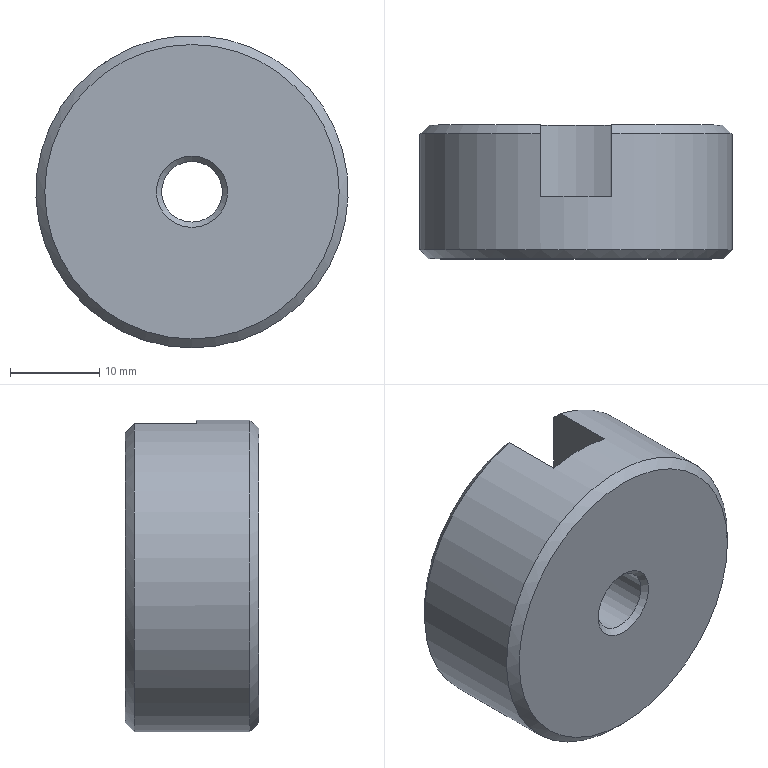Part | STEP file | 冲床-300配套压波_id598_x_t | 1 solid | 12 faces | box 35 x 15 x 35 mm | volume 11277 mm3 | plane 5 | cone 4 | cylinder 3 | commonest cylinder face diameters 6.8 x1 19 x1 35 x1
STEP:
#1=CARTESIAN_POINT('',(1396.,-127.,88.7));
#2=VERTEX_POINT('',#1);
#3=CARTESIAN_POINT('',(1388.,-127.,88.7));
#4=VERTEX_POINT('',#3);
#5=CARTESIAN_POINT('',(1392.,-127.,80.083));
#6=DIRECTION('',(0.,1.,0.));
#7=DIRECTION('',(0.,0.,-1.));
#8=AXIS2_PLACEMENT_3D('',#5,#6,#7);
#9=CIRCLE('',#8,9.5);
#10=EDGE_CURVE('',#2,#4,#9,.T.);
#11=ORIENTED_EDGE('',*,*,#10,.T.);
#12=CARTESIAN_POINT('',(1388.,-135.,88.7));
#13=VERTEX_POINT('',#12);
#14=CARTESIAN_POINT('',(1388.,-140.,88.7));
#15=DIRECTION('',(0.,-1.,0.));
#16=VECTOR('',#15,1.);
#17=LINE('',#14,#16);
#18=EDGE_CURVE('',#4,#13,#17,.T.);
#19=ORIENTED_EDGE('',*,*,#18,.T.);
#20=CARTESIAN_POINT('',(1396.,-135.,88.7));
#21=VERTEX_POINT('',#20);
#22=CARTESIAN_POINT('',(1392.,-135.,80.083));
#23=DIRECTION('',(0.,-1.,0.));
#24=DIRECTION('',(0.,0.,-1.));
#25=AXIS2_PLACEMENT_3D('',#22,#23,#24);
#26=CIRCLE('',#25,9.5);
#27=EDGE_CURVE('',#13,#21,#26,.T.);
#28=ORIENTED_EDGE('',*,*,#27,.T.);
#29=CARTESIAN_POINT('',(1396.,-140.,88.7));
#30=DIRECTION('',(0.,1.,0.));
#31=VECTOR('',#30,1.);
#32=LINE('',#29,#31);
#33=EDGE_CURVE('',#21,#2,#32,.T.);
#34=ORIENTED_EDGE('',*,*,#33,.T.);
#35=EDGE_LOOP('',(#11,#19,#28,#34));
#36=FACE_OUTER_BOUND('',#35,.T.);
#37=CARTESIAN_POINT('',(1392.,-140.,80.083));
#38=DIRECTION('',(0.,1.,0.));
#39=DIRECTION('',(-1.,0.,0.));
#40=AXIS2_PLACEMENT_3D('',#37,#38,#39);
#41=CYLINDRICAL_SURFACE('',#40,9.5);
#42=ADVANCED_FACE('',(#36),#41,.F.);
#43=CARTESIAN_POINT('',(1392.,-141.,62.583));
#44=VERTEX_POINT('',#43);
#45=CARTESIAN_POINT('',(1392.,-141.,80.083));
#46=DIRECTION('',(0.,1.,0.));
#47=DIRECTION('',(0.,0.,-1.));
#48=AXIS2_PLACEMENT_3D('',#45,#46,#47);
#49=CIRCLE('',#48,17.5);
#50=EDGE_CURVE('',#44,#44,#49,.T.);
#51=ORIENTED_EDGE('',*,*,#50,.T.);
#52=EDGE_LOOP('',(#51));
#53=FACE_BOUND('',#52,.T.);
#54=CARTESIAN_POINT('',(1388.,-128.,97.12));
#55=VERTEX_POINT('',#54);
#56=CARTESIAN_POINT('',(1388.,-135.,97.12));
#57=VERTEX_POINT('',#56);
#58=CARTESIAN_POINT('',(1388.,-142.,97.12));
#59=DIRECTION('',(0.,-1.,0.));
#60=VECTOR('',#59,1.);
#61=LINE('',#58,#60);
#62=EDGE_CURVE('',#55,#57,#61,.T.);
#63=ORIENTED_EDGE('',*,*,#62,.F.);
#64=CARTESIAN_POINT('',(1396.,-128.,97.12));
#65=VERTEX_POINT('',#64);
#66=CARTESIAN_POINT('',(1392.,-128.,80.083));
#67=DIRECTION('',(0.,-1.,0.));
#68=DIRECTION('',(0.,0.,-1.));
#69=AXIS2_PLACEMENT_3D('',#66,#67,#68);
#70=CIRCLE('',#69,17.5);
#71=EDGE_CURVE('',#55,#65,#70,.T.);
#72=ORIENTED_EDGE('',*,*,#71,.T.);
#73=CARTESIAN_POINT('',(1396.,-135.,97.12));
#74=VERTEX_POINT('',#73);
#75=CARTESIAN_POINT('',(1396.,-142.,97.12));
#76=DIRECTION('',(0.,1.,0.));
#77=VECTOR('',#76,1.);
#78=LINE('',#75,#77);
#79=EDGE_CURVE('',#74,#65,#78,.T.);
#80=ORIENTED_EDGE('',*,*,#79,.F.);
#81=CARTESIAN_POINT('',(1392.,-135.,80.083));
#82=DIRECTION('',(0.,-1.,0.));
#83=DIRECTION('',(0.,0.,1.));
#84=AXIS2_PLACEMENT_3D('',#81,#82,#83);
#85=CIRCLE('',#84,17.5);
#86=EDGE_CURVE('',#74,#57,#85,.T.);
#87=ORIENTED_EDGE('',*,*,#86,.T.);
#88=EDGE_LOOP('',(#63,#72,#80,#87));
#89=FACE_BOUND('',#88,.T.);
#90=CARTESIAN_POINT('',(1392.,-142.,80.083));
#91=DIRECTION('',(0.,1.,0.));
#92=DIRECTION('',(0.,0.,1.));
#93=AXIS2_PLACEMENT_3D('',#90,#91,#92);
#94=CYLINDRICAL_SURFACE('',#93,17.5);
#95=ADVANCED_FACE('',(#53,#89),#94,.T.);
#96=CARTESIAN_POINT('',(1396.,-127.,96.091));
#97=VERTEX_POINT('',#96);
#98=CARTESIAN_POINT('',(1396.,-127.,80.083));
#99=DIRECTION('',(0.,0.,1.));
#100=VECTOR('',#99,1.);
#101=LINE('',#98,#100);
#102=EDGE_CURVE('',#2,#97,#101,.T.);
#103=ORIENTED_EDGE('',*,*,#102,.T.);
#104=CARTESIAN_POINT('',(1388.,-127.,96.091));
#105=VERTEX_POINT('',#104);
#106=CARTESIAN_POINT('',(1392.,-127.,80.083));
#107=DIRECTION('',(0.,1.,0.));
#108=DIRECTION('',(0.,0.,-1.));
#109=AXIS2_PLACEMENT_3D('',#106,#107,#108);
#110=CIRCLE('',#109,16.5);
#111=EDGE_CURVE('',#97,#105,#110,.T.);
#112=ORIENTED_EDGE('',*,*,#111,.T.);
#113=CARTESIAN_POINT('',(1388.,-127.,80.083));
#114=DIRECTION('',(0.,0.,1.));
#115=VECTOR('',#114,1.);
#116=LINE('',#113,#115);
#117=EDGE_CURVE('',#4,#105,#116,.T.);
#118=ORIENTED_EDGE('',*,*,#117,.F.);
#119=ORIENTED_EDGE('',*,*,#10,.F.);
#120=EDGE_LOOP('',(#103,#112,#118,#119));
#121=FACE_OUTER_BOUND('',#120,.T.);
#122=CARTESIAN_POINT('',(1392.,-127.,80.083));
#123=DIRECTION('',(0.,-1.,0.));
#124=DIRECTION('',(0.,0.,-1.));
#125=AXIS2_PLACEMENT_3D('',#122,#123,#124);
#126=PLANE('',#125);
#127=ADVANCED_FACE('',(#121),#126,.F.);
#128=ORIENTED_EDGE('',*,*,#27,.F.);
#129=CARTESIAN_POINT('',(1388.,-135.,100.583));
#130=DIRECTION('',(0.,0.,-1.));
#131=VECTOR('',#130,1.);
#132=LINE('',#129,#131);
#133=EDGE_CURVE('',#57,#13,#132,.T.);
#134=ORIENTED_EDGE('',*,*,#133,.F.);
#135=ORIENTED_EDGE('',*,*,#86,.F.);
#136=CARTESIAN_POINT('',(1396.,-135.,100.583));
#137=DIRECTION('',(0.,0.,-1.));
#138=VECTOR('',#137,1.);
#139=LINE('',#136,#138);
#140=EDGE_CURVE('',#74,#21,#139,.T.);
#141=ORIENTED_EDGE('',*,*,#140,.T.);
#142=EDGE_LOOP('',(#128,#134,#135,#141));
#143=FACE_BOUND('',#142,.T.);
#144=CARTESIAN_POINT('',(1392.,-135.,76.083));
#145=VERTEX_POINT('',#144);
#146=CARTESIAN_POINT('',(1392.,-135.,80.083));
#147=DIRECTION('',(0.,-1.,0.));
#148=DIRECTION('',(0.,0.,-1.));
#149=AXIS2_PLACEMENT_3D('',#146,#147,#148);
#150=CIRCLE('',#149,4.);
#151=EDGE_CURVE('',#145,#145,#150,.T.);
#152=ORIENTED_EDGE('',*,*,#151,.T.);
#153=EDGE_LOOP('',(#152));
#154=FACE_BOUND('',#153,.T.);
#155=CARTESIAN_POINT('',(1392.,-135.,80.083));
#156=DIRECTION('',(0.,-1.,0.));
#157=DIRECTION('',(0.,0.,-1.));
#158=AXIS2_PLACEMENT_3D('',#155,#156,#157);
#159=PLANE('',#158);
#160=ADVANCED_FACE('',(#143,#154),#159,.F.);
#161=CARTESIAN_POINT('',(1392.,-142.,63.583));
#162=VERTEX_POINT('',#161);
#163=CARTESIAN_POINT('',(1392.,-142.,80.083));
#164=DIRECTION('',(0.,-1.,0.));
#165=DIRECTION('',(0.,0.,-1.));
#166=AXIS2_PLACEMENT_3D('',#163,#164,#165);
#167=CIRCLE('',#166,16.5);
#168=EDGE_CURVE('',#162,#162,#167,.T.);
#169=ORIENTED_EDGE('',*,*,#168,.T.);
#170=EDGE_LOOP('',(#169));
#171=FACE_BOUND('',#170,.T.);
#172=CARTESIAN_POINT('',(1392.,-142.,76.083));
#173=VERTEX_POINT('',#172);
#174=CARTESIAN_POINT('',(1392.,-142.,80.083));
#175=DIRECTION('',(0.,1.,0.));
#176=DIRECTION('',(0.,0.,-1.));
#177=AXIS2_PLACEMENT_3D('',#174,#175,#176);
#178=CIRCLE('',#177,4.);
#179=EDGE_CURVE('',#173,#173,#178,.T.);
#180=ORIENTED_EDGE('',*,*,#179,.T.);
#181=EDGE_LOOP('',(#180));
#182=FACE_BOUND('',#181,.T.);
#183=CARTESIAN_POINT('',(1392.,-142.,80.083));
#184=DIRECTION('',(0.,-1.,0.));
#185=DIRECTION('',(0.,0.,-1.));
#186=AXIS2_PLACEMENT_3D('',#183,#184,#185);
#187=PLANE('',#186);
#188=ADVANCED_FACE('',(#171,#182),#187,.T.);
#189=CARTESIAN_POINT('',(1392.,-141.4,76.683));
#190=VERTEX_POINT('',#189);
#191=CARTESIAN_POINT('',(1392.,-141.4,80.083));
#192=DIRECTION('',(0.,-1.,0.));
#193=DIRECTION('',(0.,0.,-1.));
#194=AXIS2_PLACEMENT_3D('',#191,#192,#193);
#195=CIRCLE('',#194,3.4);
#196=EDGE_CURVE('',#190,#190,#195,.T.);
#197=ORIENTED_EDGE('',*,*,#196,.T.);
#198=EDGE_LOOP('',(#197));
#199=FACE_BOUND('',#198,.T.);
#200=CARTESIAN_POINT('',(1392.,-135.6,76.683));
#201=VERTEX_POINT('',#200);
#202=CARTESIAN_POINT('',(1392.,-135.6,80.083));
#203=DIRECTION('',(0.,1.,0.));
#204=DIRECTION('',(0.,0.,-1.));
#205=AXIS2_PLACEMENT_3D('',#202,#203,#204);
#206=CIRCLE('',#205,3.4);
#207=EDGE_CURVE('',#201,#201,#206,.T.);
#208=ORIENTED_EDGE('',*,*,#207,.T.);
#209=EDGE_LOOP('',(#208));
#210=FACE_BOUND('',#209,.T.);
#211=CARTESIAN_POINT('',(1392.,-135.,80.083));
#212=DIRECTION('',(0.,-1.,0.));
#213=DIRECTION('',(0.,0.,-1.));
#214=AXIS2_PLACEMENT_3D('',#211,#212,#213);
#215=CYLINDRICAL_SURFACE('',#214,3.4);
#216=ADVANCED_FACE('',(#199,#210),#215,.F.);
#217=ORIENTED_EDGE('',*,*,#207,.F.);
#218=EDGE_LOOP('',(#217));
#219=FACE_BOUND('',#218,.T.);
#220=ORIENTED_EDGE('',*,*,#151,.F.);
#221=EDGE_LOOP('',(#220));
#222=FACE_BOUND('',#221,.T.);
#223=CARTESIAN_POINT('',(1392.,-135.,80.083));
#224=DIRECTION('',(0.,1.,0.));
#225=DIRECTION('',(0.,0.,1.));
#226=AXIS2_PLACEMENT_3D('',#223,#224,#225);
#227=CONICAL_SURFACE('',#226,4.,45.);
#228=ADVANCED_FACE('',(#219,#222),#227,.F.);
#229=ORIENTED_EDGE('',*,*,#179,.F.);
#230=EDGE_LOOP('',(#229));
#231=FACE_BOUND('',#230,.T.);
#232=ORIENTED_EDGE('',*,*,#196,.F.);
#233=EDGE_LOOP('',(#232));
#234=FACE_BOUND('',#233,.T.);
#235=CARTESIAN_POINT('',(1392.,-141.4,80.083));
#236=DIRECTION('',(0.,-1.,0.));
#237=DIRECTION('',(0.,0.,-1.));
#238=AXIS2_PLACEMENT_3D('',#235,#236,#237);
#239=CONICAL_SURFACE('',#238,3.4,45.);
#240=ADVANCED_FACE('',(#231,#234),#239,.F.);
#241=ORIENTED_EDGE('',*,*,#117,.T.);
#242=CARTESIAN_POINT('',(1388.,-127.,96.091));
#243=CARTESIAN_POINT('',(1388.,-127.333,96.435));
#244=CARTESIAN_POINT('',(1388.,-127.666,96.778));
#245=CARTESIAN_POINT('',(1388.,-128.,97.12));
#246=B_SPLINE_CURVE_WITH_KNOTS('',3,(#242,#243,#244,#245),.UNSPECIFIED.,.F.,.F.,(4,4),(0.,1.),.UNSPECIFIED.);
#247=EDGE_CURVE('',#105,#55,#246,.T.);
#248=ORIENTED_EDGE('',*,*,#247,.T.);
#249=ORIENTED_EDGE('',*,*,#62,.T.);
#250=ORIENTED_EDGE('',*,*,#133,.T.);
#251=ORIENTED_EDGE('',*,*,#18,.F.);
#252=EDGE_LOOP('',(#241,#248,#249,#250,#251));
#253=FACE_OUTER_BOUND('',#252,.T.);
#254=CARTESIAN_POINT('',(1388.,-116.,100.583));
#255=DIRECTION('',(1.,0.,0.));
#256=DIRECTION('',(0.,0.,-1.));
#257=AXIS2_PLACEMENT_3D('',#254,#255,#256);
#258=PLANE('',#257);
#259=ADVANCED_FACE('',(#253),#258,.T.);
#260=ORIENTED_EDGE('',*,*,#79,.T.);
#261=CARTESIAN_POINT('',(1396.,-128.,97.12));
#262=CARTESIAN_POINT('',(1396.,-127.666,96.778));
#263=CARTESIAN_POINT('',(1396.,-127.333,96.435));
#264=CARTESIAN_POINT('',(1396.,-127.,96.091));
#265=B_SPLINE_CURVE_WITH_KNOTS('',3,(#261,#262,#263,#264),.UNSPECIFIED.,.F.,.F.,(4,4),(0.,1.),.UNSPECIFIED.);
#266=EDGE_CURVE('',#65,#97,#265,.T.);
#267=ORIENTED_EDGE('',*,*,#266,.T.);
#268=ORIENTED_EDGE('',*,*,#102,.F.);
#269=ORIENTED_EDGE('',*,*,#33,.F.);
#270=ORIENTED_EDGE('',*,*,#140,.F.);
#271=EDGE_LOOP('',(#260,#267,#268,#269,#270));
#272=FACE_OUTER_BOUND('',#271,.T.);
#273=CARTESIAN_POINT('',(1396.,-135.,100.583));
#274=DIRECTION('',(-1.,0.,0.));
#275=DIRECTION('',(0.,-1.,0.));
#276=AXIS2_PLACEMENT_3D('',#273,#274,#275);
#277=PLANE('',#276);
#278=ADVANCED_FACE('',(#272),#277,.T.);
#279=ORIENTED_EDGE('',*,*,#50,.F.);
#280=EDGE_LOOP('',(#279));
#281=FACE_BOUND('',#280,.T.);
#282=ORIENTED_EDGE('',*,*,#168,.F.);
#283=EDGE_LOOP('',(#282));
#284=FACE_BOUND('',#283,.T.);
#285=CARTESIAN_POINT('',(1392.,-142.,80.083));
#286=DIRECTION('',(0.,1.,0.));
#287=DIRECTION('',(0.,0.,1.));
#288=AXIS2_PLACEMENT_3D('',#285,#286,#287);
#289=CONICAL_SURFACE('',#288,16.5,45.);
#290=ADVANCED_FACE('',(#281,#284),#289,.T.);
#291=ORIENTED_EDGE('',*,*,#247,.F.);
#292=ORIENTED_EDGE('',*,*,#111,.F.);
#293=ORIENTED_EDGE('',*,*,#266,.F.);
#294=ORIENTED_EDGE('',*,*,#71,.F.);
#295=EDGE_LOOP('',(#291,#292,#293,#294));
#296=FACE_OUTER_BOUND('',#295,.T.);
#297=CARTESIAN_POINT('',(1392.,-128.,80.083));
#298=DIRECTION('',(0.,-1.,0.));
#299=DIRECTION('',(0.,0.,-1.));
#300=AXIS2_PLACEMENT_3D('',#297,#298,#299);
#301=CONICAL_SURFACE('',#300,17.5,45.);
#302=ADVANCED_FACE('',(#296),#301,.T.);
#303=CLOSED_SHELL('',(#42,#95,#127,#160,#188,#216,#228,#240,#259,#278,#290,#302));
#304=MANIFOLD_SOLID_BREP('',#303);
#305=(LENGTH_UNIT()NAMED_UNIT(*)SI_UNIT(.MILLI.,.METRE.));
#306=UNCERTAINTY_MEASURE_WITH_UNIT(LENGTH_MEASURE(0.0508),#305,'','');
#307=(NAMED_UNIT(*)PLANE_ANGLE_UNIT()SI_UNIT($,.RADIAN.));
#308=PLANE_ANGLE_MEASURE_WITH_UNIT(PLANE_ANGLE_MEASURE(0.01745),#307);
#309=DIMENSIONAL_EXPONENTS(0.,0.,0.,0.,0.,0.,0.);
#310=(CONVERSION_BASED_UNIT('DEGREE',#308)NAMED_UNIT(#309)PLANE_ANGLE_UNIT());
#311=(NAMED_UNIT(*)SI_UNIT($,.STERADIAN.)SOLID_ANGLE_UNIT());
#312=(GEOMETRIC_REPRESENTATION_CONTEXT(3)GLOBAL_UNCERTAINTY_ASSIGNED_CONTEXT((#306))GLOBAL_UNIT_ASSIGNED_CONTEXT((#305,#310,#311))REPRESENTATION_CONTEXT('',''));
#313=ADVANCED_BREP_SHAPE_REPRESENTATION('',(#304),#312);